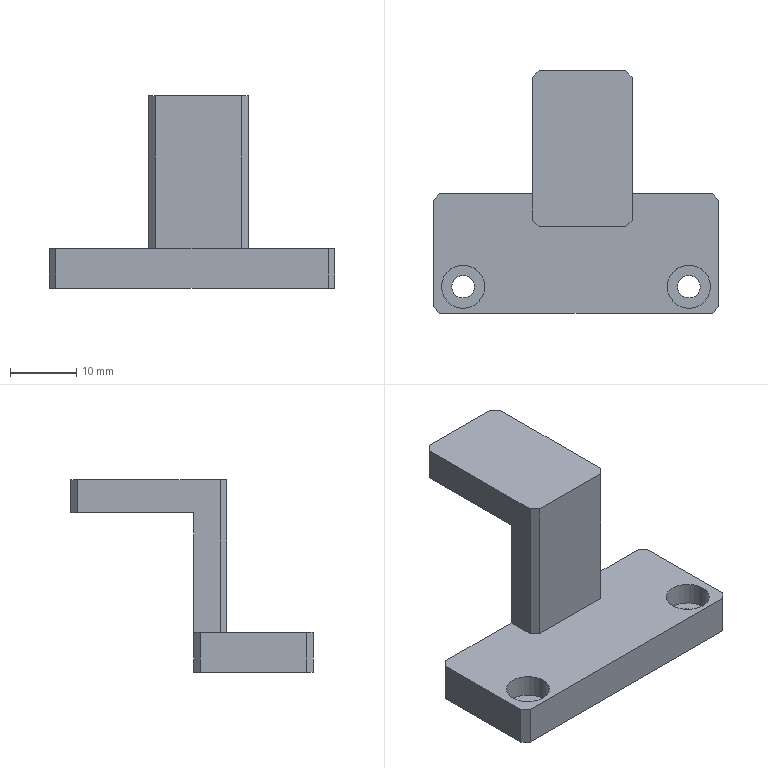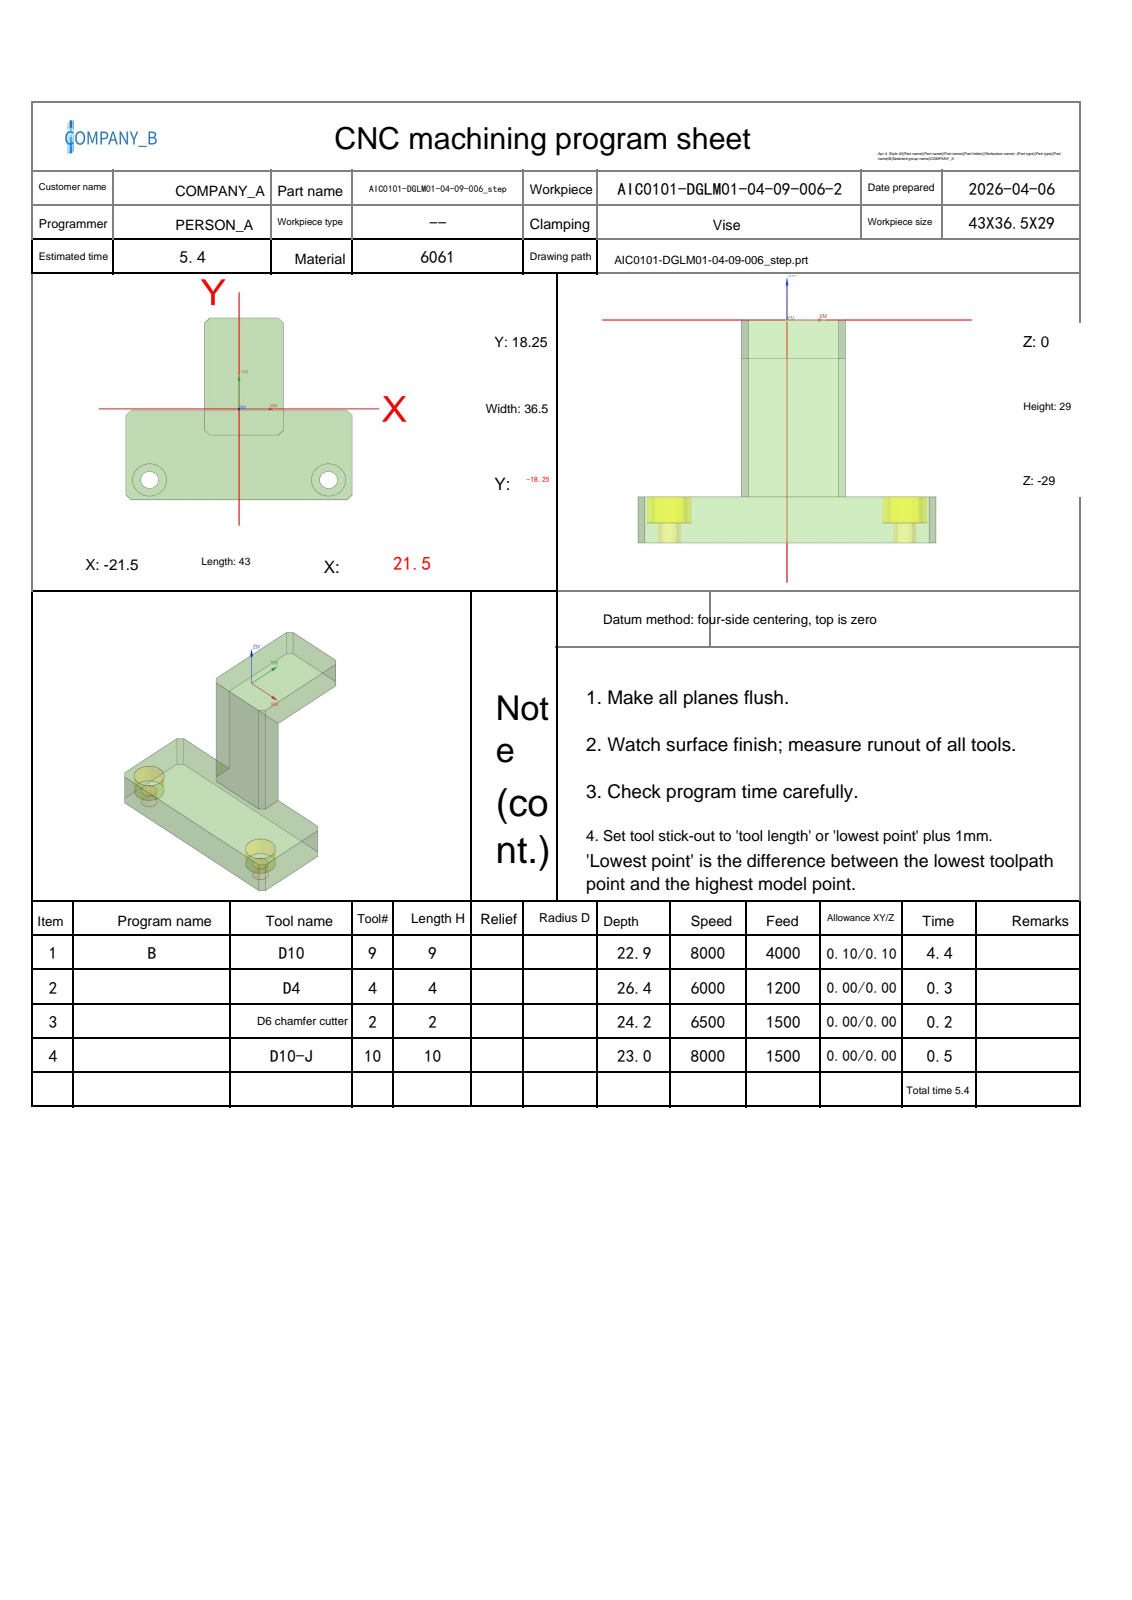NC program | NX | posted by the shop | part box 43 x 36.5 x 29 mm
Lines 1 to 972 of 4586:
%
O0001
(Machine time: 6.22 MIN)
(===Total Tool:4===)
(T9=D10     D=10.  R=0.   D-  H09 Z=-22.9 )
(T4=D4      D=4.   R=0.   D-  H04 Z=-26.4 )
(T2=D6 chamfer cutter   D=6.   R=0.   D-  H02 Z=-24.2 )
(T10=D10-J  D=10.  R=0.   D10 H10 Z=-23.  )
G80 G90 G17 G49 G40
G91 G28 Z0
M01
N1 T09 M06
(D10  D=10. R=0. H=09 ce=0.25 di=0.10)
G00 G90 G54 X-35.099 Y-10.332 M03 S8000
G43 H09 Z20.
M08
Z2.1
G01 X-35.001 Y-10.314 Z1.476 F4000.
X-34.903 Y-10.296 Z1.228
X-34.804 Y-10.278 Z1.046
X-34.706 Y-10.26 Z.9
X-34.607 Y-10.242 Z.777
X-34.509 Y-10.224 Z.672
X-34.411 Y-10.206 Z.58
X-34.312 Y-10.188 Z.5
X-34.214 Y-10.17 Z.43
X-34.116 Y-10.152 Z.368
X-34.017 Y-10.134 Z.314
X-33.919 Y-10.116 Z.267
X-33.82 Y-10.098 Z.227
X-33.722 Y-10.08 Z.192
X-33.624 Y-10.062 Z.164
X-33.525 Y-10.044 Z.14
X-33.427 Y-10.027 Z.123
X-33.329 Y-10.009 Z.11
X-33.23 Y-9.991 Z.103
X-33.132 Y-9.973 Z.1
X-30.88 Y-9.561
G03 X-30.51 Y-9.27 I-.096 J.503
X-29.9 Y-6.027 I-9.761 J3.513
X-29.692 Y2.334 I-167.742 J8.361
X-29.702 Y4.201 I-167.951 J0.0
G02 X-29.723 Y9.588 I703.046 J5.387
X-29.664 Y18.677 I703.067 J0.0
X-25.831 Y24.268 I6.588 J-.408
X-19.878 Y25.71 I6.684 J-14.582
X-11.771 Y25.954 I8.107 J-135.053
X-10.284 Y25.945 I0.0 J-135.296
G01 X22.13 Y25.932
G02 X28.067 Y21.993 I-.133 J-6.643
X29.449 Y16.271 I-14.607 J-6.557
X29.713 Y7.575 I-143.052 J-8.695
X29.698 Y5.476 I-143.316 J0.0
G01 X29.681 Y-18.42
G02 X25.869 Y-24.247 I-6.599 J.158
X20.079 Y-25.692 I-6.608 J14.146
X11.869 Y-25.956 I-8.21 J127.869
X10.245 Y-25.945 I0.0 J128.132
G01 X-22.171 Y-25.93
G02 X-28.026 Y-22.061 I.169 J6.619
X-29.462 Y-16.11 I14.613 J6.676
X-29.614 Y-12.83 I35.28 J3.28
X-29.302 Y-8.137 I35.432 J0.0
G03 X-28.904 Y2.261 I-135.723 J10.398
X-28.91 Y3.491 I-136.121 J0.0
G02 X-28.922 Y7.625 I709.413 J4.134
X-28.863 Y16.738 I709.425 J0.0
X-24.741 Y22.947 I7.759 J-.678
X-18.641 Y24.75 I7.505 J-14.175
X-10.084 Y25.147 I8.556 J-91.966
X-8.813 Y25.138 I0.0 J-92.364
G01 X20.207 Y25.129
G02 X26.68 Y21.024 I-.379 J-7.754
X28.524 Y14.687 I-14.343 J-7.61
X28.906 Y5.741 I-104.616 J-8.946
X28.893 Y4.059 I-104.998 J0.0
G01 X28.882 Y-16.417
G02 X24.804 Y-22.91 I-7.753 J.342
X18.39 Y-24.779 I-7.66 J14.347
X9.425 Y-25.156 I-8.965 J106.528
X7.761 Y-25.143 I0.0 J106.905
G01 X-20.167 Y-25.131
G02 X-26.629 Y-21.102 I.341 J7.744
X-28.535 Y-14.46 I14.057 J7.628
X-28.605 Y-11.776 I51.743 J2.683
X-28.407 Y-7.251 I51.812 J0.0
G03 X-28.081 Y7.217 I-320.735 J14.467
X-28.101 Y10.838 I-321.061 J0.0
G02 X-28.126 Y12.212 I38.122 J1.374
X-27.974 Y15.613 I38.147 J0.0
X-23.079 Y22.154 I8.78 J-1.468
X-16.395 Y23.964 I8.13 J-16.776
X-7.027 Y24.352 I9.368 J-112.703
X-5.446 Y24.341 I0.0 J-113.092
G01 X18.294 Y24.327
G02 X25.851 Y19.431 I-.359 J-8.835
X27.7 Y12.764 I-16.412 J-8.143
X28.105 Y3.246 I-111.872 J-9.518
X28.092 Y1.576 I-112.276 J0.0
X28.118 Y-5.22 I-878.703 J-6.795
X28.067 Y-14.723 I-878.729 J0.0
X23.208 Y-22.083 I-8.816 J.536
X16.623 Y-23.937 I-8.116 J16.208
X7.487 Y-24.347 I-9.136 J101.66
X6.156 Y-24.338 I0.0 J102.07
G01 X-18.144 Y-24.333
G02 X-25.822 Y-19.476 I.219 J8.843
X-27.593 Y-12.229 I14.676 J7.426
X-27.611 Y-10.065 I128.798 J2.164
X-27.441 Y-3.447 I128.816 J0.0
G03 X-27.276 Y12.759 I-867.03 J16.931
G02 X-21.723 Y21.294 I9.672 J-.219
X-14.557 Y23.163 I8.645 J-18.474
X-4.967 Y23.548 I9.59 J-119.225
X-3.528 Y23.539 I0.0 J-119.61
G01 X16.532 Y23.523
G02 X25.055 Y17.953 I-.24 J-9.674
X26.881 Y11.109 I-18.139 J-8.505
X27.3 Y1.375 I-112.809 J-9.735
X27.289 Y-.158 I-113.228 J0.0
X27.307 Y-5.158 I-719.586 J-4.999
X27.265 Y-12.938 I-719.603 J0.0
X21.676 Y-21.318 I-9.667 J.393
X14.669 Y-23.151 I-8.567 J18.443
X5.031 Y-23.548 I-9.638 J116.603
X3.561 Y-23.539 I0.0 J117.
G01 X-16.259 Y-23.534
X-16.273
G02 X-25.201 Y-17.597 I0.0 J9.682
X-26.646 Y-10.669 I17.356 J7.235
X-26.685 Y-6.775 I195.538 J3.894
X-26.569 Y-.062 I195.577 J0.0
X-26.455 Y11.482 I890.841 J-3.088
X-20.487 Y20.435 I10.294 J-.397
X-13.408 Y22.308 I8.863 J-19.183
X-3.331 Y22.748 I10.076 J-115.189
X-1.821 Y22.738 I0.0 J-115.629
X5.249 Y22.767 I7.07 J-872.675
X15.038 Y22.712 I0.0 J-872.703
X24.267 Y16.57 I-.229 J-10.348
X26.096 Y9.315 I-20.036 J-8.91
X26.496 Y-.533 I-121.222 J-9.847
X26.488 Y-1.874 I-121.622 J0.0
X26.517 Y-5.594 I-238.869 J-3.72
X26.441 Y-11.633 I-238.898 J0.0
X20.365 Y-20.493 I-10.296 J.547
X12.873 Y-22.365 I-9.019 J20.176
X3.265 Y-22.742 I-9.608 J122.293
X2.164 Y-22.737 I0.0 J122.67
X-5.189 Y-22.767 I-7.352 J884.922
X-15.016 Y-22.713 I0.0 J884.953
X-24.356 Y-16.185 I.158 J10.172
X-25.751 Y-8.916 I20.041 J7.614
X-25.817 Y-3.574 I217.316 J5.341
X-25.743 Y2.076 I217.381 J0.0
X-25.745 Y3.097 I237.464 J1.02
X-25.639 Y10.209 I237.467 J0.0
X-19.185 Y19.649 I10.846 J-.489
X-11.532 Y21.546 I9.29 J-21.093
X-1.516 Y21.942 I10.015 J-126.302
X-.262 Y21.936 I0.0 J-126.699
X5.345 Y21.967 I5.607 J-504.237
X13.717 Y21.898 I0.0 J-504.268
X23.33 Y15.576 I-.237 J-10.831
X25.263 Y8.097 I-20.328 J-9.243
X25.695 Y-2.142 I-121.077 J-10.24
X25.687 Y-3.57 I-121.509 J0.0
X25.716 Y-5.906 I-93.971 J-2.336
X25.598 Y-10.608 I-94. J0.0
X19.283 Y-19.599 I-10.758 J.843
X11.718 Y-21.526 I-9.272 J20.586
X1.596 Y-21.944 I-10.122 J122.471
X.29 Y-21.937 I0.0 J122.889
X-5.352 Y-21.971 I-5.642 J461.8
X-13.769 Y-21.894 I0.0 J461.834
X-23.383 Y-15.145 I.225 J10.543
X-24.839 Y-8.041 I20.527 J7.907
X-24.983 Y-1.004 I171.254 J7.037
X-24.934 Y3.106 I171.399 J0.0
X-24.945 Y4.407 I78.052 J1.301
X-24.779 Y9.493 I78.063 J0.0
X-18.144 Y18.768 I11.205 J-1.005
X-10.583 Y20.695 I9.454 J-21.297
X-.124 Y21.143 I10.459 J-121.839
X1.244 Y21.135 I0.0 J-122.287
X5.457 Y21.162 I4.213 J-334.395
X12.363 Y21.091 I0.0 J-334.422
X20.144 Y17.822 I-.204 J-11.382
X23.766 Y10.832 I-10.854 J-10.057
X24.783 Y1.624 I-44.86 J-9.611
X24.898 Y-4.053 I-139.858 J-5.677
X24.81 Y-9.014 I-139.973 J0.0
X18.124 Y-18.775 I-11.253 J.538
X10.323 Y-20.722 I-9.548 J21.645
X-.202 Y-21.145 I-10.525 J130.707
X-1.665 Y-21.137 I0.0 J131.13
X-5.681 Y-21.166 I-4.016 J280.073
X-12.464 Y-21.084 I0.0 J280.102
X-19.777 Y-18.098 I.247 J11.055
X-23.319 Y-11.371 I9.676 J9.39
X-24.126 Y-3.277 I40.22 J8.094
X-24.123 Y-2.784 I41.026 J0.0
X-24.159 Y.812 I179.52 J3.597
X-24.027 Y7.673 I179.556 J0.0
X-19.342 Y16.576 I11.625 J-.434
X-12.27 Y19.446 I9.931 J-14.322
X-2.397 Y20.273 I9.913 J-58.987
X4.527 Y20.359 I6.924 J-277.627
X11.122 Y20.281 I0.0 J-277.713
X18.549 Y17.514 I-.247 J-12.017
X22.677 Y10.666 I-9.496 J-10.391
X23.917 Y1.813 I-37.219 J-9.726
X24.074 Y-3.664 I-95.415 J-5.477
X23.978 Y-7.942 I-95.573 J0.0
X17.054 Y-17.93 I-11.608 J.654
X9.251 Y-19.892 I-9.705 J22.092
X-1.267 Y-20.339 I-10.518 J123.549
X-2.496 Y-20.333 I0.0 J123.996
X-5.605 Y-20.36 I-3.11 J178.005
X-11.294 Y-20.269 I0.0 J178.033
X-18.637 Y-17.327 I.323 J11.44
X-22.346 Y-10.607 I9.587 J9.674
X-23.277 Y-2.129 I38.123 J8.478
G01 Y-2.036
G02 X-23.338 Y1.46 I99.559 J3.496
X-23.197 Y6.76 I99.621 J0.0
X-15.895 Y17.151 I12.014 J-.682
X-8. Y19.088 I9.877 J-23.198
X2.785 Y19.539 I10.785 J-128.663
X4.067 Y19.533 I0.0 J-129.115
X6.025 Y19.561 I1.958 J-68.354
X10.942 Y19.384 I0.0 J-68.382
X20.81 Y12.331 I-1.038 J-11.884
X22.824 Y4.381 I-22.519 J-9.935
X23.23 Y-3.317 I-72.836 J-7.699
X23.147 Y-6.803 I-73.242 J0.0
X15.953 Y-17.119 I-11.932 J.655
X7.751 Y-19.113 I-10.029 J23.382
X-3.155 Y-19.543 I-10.905 J138.046
X-4.638 Y-19.535 I0.0 J138.476
X-6.396 Y-19.565 I-1.758 J52.38
X-11.349 Y-19.33 I0.0 J52.409
X-20.515 Y-12.319 I1.4 J11.327
X-22.266 Y-4.388 I22.554 J9.139
X-22.504 Y1.323 I68.472 J5.711
X-22.344 Y6.002 I68.709 J0.0
X-15.122 Y16.202 I12.194 J-.977
X-7.098 Y18.251 I10.109 J-22.851
X4.217 Y18.743 I11.315 J-129.888
X6.007 Y18.731 I0.0 J-130.38
X6.856 Y18.746 I.849 J-23.129
X12.197 Y18.122 I0.0 J-23.144
X19.962 Y11.346 I-3.378 J-11.707
X22.014 Y3.24 I-23.024 J-10.141
X22.372 Y-2.804 I-50.768 J-6.044
X22.265 Y-6.104 I-51.126 J0.0
X15.188 Y-16.162 I-12.056 J.964
X7.006 Y-18.261 I-10.19 J22.724
X-4.228 Y-18.743 I-11.233 J130.707
X-6.02 Y-18.73 I0.0 J131.189
X-6.851 Y-18.746 I-.831 J22.555
X-12.052 Y-18.138 I0.0 J22.571
X-19.617 Y-11.346 I3.255 J11.234
X-21.391 Y-3.663 I22.516 J9.245
X-21.643 Y1.253 I47.658 J4.916
X-21.48 Y5.204 I47.91 J0.0
X-14.139 Y15.365 I12.368 J-1.203
X-5.959 Y17.445 I10.291 J-23.354
X3.731 Y17.909 I9.689 J-100.918
X8.025 Y17.818 I0.0 J-101.382
X15.743 Y14.883 I-.511 J-12.961
X20.159 Y7.634 I-9.99 J-11.055
X21.484 Y-2.348 I-36.948 J-9.982
X21.359 Y-5.445 I-38.272 J0.0
X14.277 Y-15.286 I-12.169 J1.288
X6.108 Y-17.427 I-10.304 J22.663
X-3.714 Y-17.908 I-9.822 J99.91
X-7.954 Y-17.819 I0.0 J100.392
X-15.568 Y-14.827 I.475 J12.39
X-19.659 Y-7.771 I9.912 J10.461
X-20.754 Y.988 I34.486 J8.758
X-20.56 Y4.691 I35.581 J0.0
X-13.38 Y14.43 I12.399 J-1.625
X-5.297 Y16.587 I10.395 J-22.731
X3.288 Y17.073 I8.585 J-75.618
X7.243 Y16.97 I0.0 J-76.104
X15.566 Y13.339 I-.659 J-12.866
X19.508 Y6.025 I-11.673 J-11.009
X20.559 Y-2.044 I-30.451 J-8.069
X20.467 Y-4.442 I-31.502 J0.0
X13.343 Y-14.43 I-12.266 J1.215
X5.34 Y-16.58 I-10.336 J22.504
X-3.264 Y-17.072 I-8.605 J75.058
X-7.119 Y-16.973 I0.0 J75.55
X-15.378 Y-13.222 I.611 J12.311
X-19.008 Y-5.979 I11.796 J10.444
X-19.822 Y.763 I27.522 J6.742
X-19.643 Y3.949 I28.336 J0.0
X-12.607 Y13.505 I12.403 J-1.764
X-4.393 Y15.76 I10.579 J-22.45
X2.907 Y16.219 I7.3 J-57.794
X6.466 Y16.11 I0.0 J-58.254
X17.471 Y8.416 I-.795 J-12.856
X19.595 Y-1.634 I-22.721 J-10.05
X19.496 Y-3.849 I-24.844 J0.0
X12.709 Y-13.427 I-12.172 J1.431
X4.669 Y-15.722 I-10.509 J21.591
X-2.814 Y-16.218 I-7.483 J56.159
X-6.426 Y-16.103 I0.0 J56.655
X-16.985 Y-8.499 I.89 J12.369
X-18.846 Y.514 I20.904 J9.013
X-18.672 Y3.321 I22.764 J0.0
X-11.746 Y12.627 I12.335 J-1.949
X-3.383 Y14.948 I10.737 J-22.464
X2.469 Y15.349 I5.852 J-42.537
X6.035 Y15.2 I0.0 J-42.938
X16.553 Y7.66 I-1.251 J-12.851
X18.578 Y-1.232 I-18.506 J-8.892
X18.464 Y-3.4 I-20.532 J0.0
X11.922 Y-12.498 I-12.014 J1.738
X3.831 Y-14.885 I-10.633 J21.134
X-2.443 Y-15.342 I-6.274 J42.853
X-5.663 Y-15.222 I0.0 J43.31
X-16.09 Y-7.637 I1.091 J12.459
X-17.813 Y.221 I17.062 J7.858
X-17.619 Y2.911 I18.785 J0.0
X-10.945 Y11.719 I12.145 J-2.271
X-2.837 Y14.077 I10.705 J-21.685
X2.074 Y14.454 I4.911 J-31.865
X5.696 Y14.25 I0.0 J-32.242
X15.747 Y6.678 I-1.787 J-12.83
X17.507 Y-.908 I-15.47 J-7.586
X17.41 Y-2.73 I-17.23 J0.0
X11.152 Y-11.555 I-11.804 J1.739
X3.089 Y-14.035 I-10.693 J20.422
X-2.002 Y-14.442 I-5.092 J31.603
X-5.283 Y-14.274 I0.0 J32.01
X-15.202 Y-6.766 I1.598 J12.417
X-16.717 Y-.075 I14.013 J6.691
X-16.472 Y2.673 I15.529 J0.0
X-10.294 Y10.72 I11.802 J-2.666
X-1.917 Y13.248 I10.825 J-20.726
X1.731 Y13.533 I3.647 J-23.19
X5.807 Y13.177 I0.0 J-23.475
X14.889 Y5.788 I-2.708 J-12.604
X16.363 Y-.467 I-12.53 J-6.255
X16.144 Y-2.934 I-14.005 J0.0
X10.318 Y-10.636 I-11.422 J2.586
X2.282 Y-13.188 I-10.653 J19.622
X-1.579 Y-13.515 I-3.861 J22.573
X-5.441 Y-13.187 I0.0 J22.901
X-14.402 Y-5.664 I2.585 J12.178
X-15.552 Y-.408 I11.441 J5.256
X-14.965 Y3.392 I12.591 J0.0
X-8.808 Y10.164 I11.459 J-4.232
X1.477 Y12.541 I10.285 J-21.074
X4.266 Y12.374 I0.0 J-23.45
X14.431 Y3.836 I-1.92 J-12.606
X15.16 Y-.086 I-10.183 J-3.922
X10.235 Y-9.209 I-10.913 J0.0
X2.043 Y-12.235 I-10.749 J16.5
X-1.244 Y-12.539 I-3.287 J17.633
X-5.497 Y-12.027 I0.0 J17.936
X-14.275 Y-.439 I3.26 J11.588
X-14.213 Y.775 I12.038 J0.0
X-9.045 Y8.606 I10.962 J-1.613
X1.189 Y11.519 I10.235 J-16.523
X3.765 Y11.348 I0.0 J-19.436
X13.808 Y.656 I-1.729 J-11.687
X13.817 Y.229 I-10.242 J-.426
X9.582 Y-8.071 I-10.251 J0.0
X.689 Y-11.391 I-10.498 J14.548
X-1.122 Y-11.517 I-1.81 J12.935
X-7.568 Y-9.815 I0.0 J13.061
X-12.912 Y-.645 I5.365 J9.268
X-8.602 Y7.326 I10.217 J-.372
X.923 Y10.433 I9.525 J-13.049
X3.471 Y10.231 I0.0 J-16.156
X11.94 Y3.058 I-1.82 J-10.736
X12.341 Y.368 I-8.818 J-2.69
X9.443 Y-6.343 I-9.219 J0.0
X.292 Y-10.333 I-10.199 J10.901
X-.936 Y-10.401 I-1.228 J11.081
X-9.056 Y-6.892 I0.0 J11.148
X-11.361 Y-.964 I6.47 J5.928
X-8.968 Y5.059 I8.775 J0.0
X.674 Y9.262 I9.642 J-8.958
X3.721 Y8.905 I0.0 J-13.161
X10.164 Y3.498 I-2.189 J-9.152
X10.705 Y.539 I-7.827 J-2.959
X8.359 Y-5.271 I-8.368 J0.0
X-.504 Y-9.135 I-8.862 J8.231
X-3.266 Y-8.816 I0.0 J12.095
X-9.231 Y-3.597 I1.892 J8.182
X-9.613 Y-1.14 I7.711 J2.457
X-7.269 Y4.557 I8.093 J0.0
X.524 Y7.955 I7.793 J-7.237
X3.921 Y7.398 I0.0 J-10.635
X8.829 Y.614 I-2.235 J-6.784
G01 Y.592
G02 X4.759 Y-6.202 I-8.392 J.412
X-.297 Y-7.736 I-5.056 J7.568
X-3.736 Y-7.061 I0.0 J9.101
X-7.557 Y-1.158 I2.649 J5.903
X-6.776 Y1.925 I6.47 J0.0
X.42 Y6.357 I7.196 J-3.626
X2.264 Y6.143 I0.0 J-8.058
X6.402 Y.697 I-1.515 J-5.446
X5.99 Y-1.421 I-5.653 J0.0
X.012 Y-5.749 I-6.145 J2.195
X-4.292 Y-1.308 I.139 J4.441
X-3.901 Y.516 I4.443 J0.0
G01 X-3.376 Y1.594
X-3.33 Y1.683 Z.103
X-3.284 Y1.772 Z.11
X-3.238 Y1.861 Z.123
X-3.192 Y1.949 Z.14
X-3.146 Y2.038 Z.164
X-3.1 Y2.127 Z.192
X-3.054 Y2.216 Z.227
X-3.008 Y2.305 Z.267
X-2.962 Y2.393 Z.314
X-2.916 Y2.482 Z.368
X-2.87 Y2.571 Z.43
X-2.824 Y2.66 Z.5
X-2.778 Y2.749 Z.58
X-2.732 Y2.837 Z.672
X-2.686 Y2.926 Z.777
X-2.64 Y3.015 Z.9
X-2.594 Y3.104 Z1.046
X-2.548 Y3.193 Z1.228
X-2.502 Y3.281 Z1.476
X-2.456 Y3.37 Z2.1
G00 Z20.
G00 G90 X-16.642 Y-26.25 M03 S8000
Z15.5
Z.913
G01 Z-.587 F4000.
Y-23.15
X-22.53
X-23.965 Y-21.715
X-26.4 Y-19.28
Y.78
X-22.53 Y4.65
X-15.949
X-15.863 Y4.653
X-15.804 Y4.589
X-15.661 Y4.444
G03 X-15.464 Y4.349 I.23 J.227
G02 X-13.22 Y1.863 I-.256 J-2.487
X-13.415 Y.894 I-2.5 J0.0
G01 X-17.755 Y-9.432
G02 X-20.06 Y-10.963 I-2.305 J.969
X-22.56 Y-8.463 I0.0 J2.5
X-22.365 Y-7.495 I2.5 J0.0
G01 X-18.025 Y2.831
G02 X-15.938 Y4.353 I2.305 J-.969
G01 X-15.86 Y4.354
X-15.81 Y4.413
X-15.674 Y4.551
G02 X-15.437 Y4.65 I.237 J-.233
G01 X-11.65
Y-6.362
X-7.662 Y-10.35
X9.562
X13.55 Y-6.362
Y4.65
X18.043
X18.087 Y4.661
X18.111 Y4.622
X18.175 Y4.557
X18.212 Y4.508
X18.274 Y4.513
G02 X20.615 Y2.433 I-.124 J-2.497
G01 X22.774 Y-10.329
G02 X22.809 Y-10.746 I-2.465 J-.417
X20.309 Y-13.246 I-2.5 J0.0
X17.844 Y-11.163 I0.0 J2.5
G01 X15.685 Y1.599
G02 X15.65 Y2.016 I2.465 J.417
X18.046 Y4.514 I2.5 J0.0
G01 X18.088 Y4.504
X18.109 Y4.542
X18.172 Y4.605
X18.214 Y4.657
X18.28 Y4.65
X22.53
X26.4 Y.78
Y-19.28
X22.53 Y-23.15
X20.502
G02 X19.554 Y-22.467 I0.0 J1.
G01 X17.457 Y-16.177
G03 X16.896 Y-15.572 I-.949 J-.317
G02 X16.283 Y-14.65 I.387 J.922
X16.575 Y-13.944 I1. J0.0
G01 X17.194 Y-13.325
G02 X17.9 Y-13.033 I.706 J-.708
X18.9 Y-14.032 I0.0 J-1.
G01 Y-14.652
G02 X18.262 Y-15.582 I-1. J.002
G03 X17.702 Y-16.129 I.363 J-.932
G01 X15.038 Y-22.535
G02 X14.115 Y-23.15 I-.923 J.385
G01 X-9.665
G02 X-10.446 Y-22.774 I0.0 J1.
G01 X-13.891 Y-18.459
X-13.947 Y-18.395
G02 X-14.635 Y-16.673 I1.812 J1.722
X-12.135 Y-14.173 I2.5 J0.0
G01 X14.035
G02 X16.535 Y-16.673 I0.0 J-2.5
X14.035 Y-19.173 I-2.5 J0.0
G01 X-9.655
G03 X-10.446 Y-19.562 I0.0 J-1.
G01 X-12.564 Y-22.307
G02 X-14.28 Y-23.15 I-1.715 J1.324
G01 X-14.39
G02 X-14.677 Y-22.962 I0.0 J.315
G01 X-17.696 Y-16.116
G03 X-18.255 Y-15.585 I-.915 J-.404
G02 X-18.9 Y-14.652 I.355 J.935
G01 Y-12.122
G02 X-17.9 Y-11.123 I1. J-.002
X-17.166 Y-11.444 I0.0 J-1.
G03 X-16.953 Y-11.666 I5.516 J5.082
G01 X-14.675 Y-13.944
G02 X-14.383 Y-14.65 I-.708 J-.706
X-15.382 Y-15.65 I-1. J0.0
G01 X-15.882
Y-26.25
Z.913
G00 X-16.642
Z.326
G01 Z-1.174
Y-23.15
X-22.53
X-23.965 Y-21.715
X-26.4 Y-19.28
Y.78
X-22.53 Y4.65
X-15.949
X-15.863 Y4.653
X-15.804 Y4.589
X-15.661 Y4.444
G03 X-15.464 Y4.349 I.23 J.227
G02 X-13.22 Y1.863 I-.256 J-2.487
X-13.415 Y.894 I-2.5 J0.0
G01 X-17.755 Y-9.432
G02 X-20.06 Y-10.963 I-2.305 J.969
X-22.56 Y-8.463 I0.0 J2.5
X-22.365 Y-7.495 I2.5 J0.0
G01 X-18.025 Y2.831
G02 X-15.938 Y4.353 I2.305 J-.969
G01 X-15.86 Y4.354
X-15.81 Y4.413
X-15.674 Y4.551
G02 X-15.437 Y4.65 I.237 J-.233
G01 X-11.65
Y-6.362
X-7.662 Y-10.35
X9.562
X13.55 Y-6.362
Y4.65
X18.043
X18.087 Y4.661
X18.111 Y4.622
X18.175 Y4.557
X18.212 Y4.508
X18.274 Y4.513
G02 X20.615 Y2.433 I-.124 J-2.497
G01 X22.774 Y-10.329
G02 X22.809 Y-10.746 I-2.465 J-.417
X20.309 Y-13.246 I-2.5 J0.0
X17.844 Y-11.163 I0.0 J2.5
G01 X15.685 Y1.599
G02 X15.65 Y2.016 I2.465 J.417
X18.046 Y4.514 I2.5 J0.0
G01 X18.088 Y4.504
X18.109 Y4.542
X18.172 Y4.605
X18.214 Y4.657
X18.28 Y4.65
X22.53
X26.4 Y.78
Y-19.28
X22.53 Y-23.15
X20.502
G02 X19.554 Y-22.467 I0.0 J1.
G01 X17.457 Y-16.177
G03 X16.896 Y-15.572 I-.949 J-.317
G02 X16.283 Y-14.65 I.387 J.922
X16.575 Y-13.944 I1. J0.0
G01 X17.194 Y-13.325
G02 X17.9 Y-13.033 I.706 J-.708
X18.9 Y-14.032 I0.0 J-1.
G01 Y-14.652
G02 X18.262 Y-15.582 I-1. J.002
G03 X17.702 Y-16.129 I.363 J-.932
G01 X15.038 Y-22.535
G02 X14.115 Y-23.15 I-.923 J.385
G01 X-9.665
G02 X-10.446 Y-22.774 I0.0 J1.
G01 X-13.891 Y-18.459
X-13.947 Y-18.395
G02 X-14.635 Y-16.673 I1.812 J1.722
X-12.135 Y-14.173 I2.5 J0.0
G01 X14.035
G02 X16.535 Y-16.673 I0.0 J-2.5
X14.035 Y-19.173 I-2.5 J0.0
G01 X-9.655
G03 X-10.446 Y-19.562 I0.0 J-1.
G01 X-12.564 Y-22.307
G02 X-14.28 Y-23.15 I-1.715 J1.324
G01 X-14.39
G02 X-14.677 Y-22.962 I0.0 J.315
G01 X-17.696 Y-16.116
G03 X-18.255 Y-15.585 I-.915 J-.404
G02 X-18.9 Y-14.652 I.355 J.935
G01 Y-12.122
G02 X-17.9 Y-11.123 I1. J-.002
X-17.166 Y-11.444 I0.0 J-1.
G03 X-16.953 Y-11.666 I5.516 J5.082
G01 X-14.675 Y-13.944
G02 X-14.383 Y-14.65 I-.708 J-.706
X-15.382 Y-15.65 I-1. J0.0
G01 X-15.882
Y-26.25
Z.326
G00 X-16.642
Z-.262
G01 Z-1.762
Y-23.15
X-22.53
X-23.965 Y-21.715
X-26.4 Y-19.28
Y.78
X-22.53 Y4.65
X-15.949
X-15.863 Y4.653
X-15.804 Y4.589
X-15.661 Y4.444
G03 X-15.464 Y4.349 I.23 J.227
G02 X-13.22 Y1.863 I-.256 J-2.487
X-13.415 Y.894 I-2.5 J0.0
G01 X-17.755 Y-9.432
G02 X-20.06 Y-10.963 I-2.305 J.969
X-22.56 Y-8.463 I0.0 J2.5
X-22.365 Y-7.495 I2.5 J0.0
G01 X-18.025 Y2.831
G02 X-15.938 Y4.353 I2.305 J-.969
G01 X-15.86 Y4.354
X-15.81 Y4.413
X-15.674 Y4.551
G02 X-15.437 Y4.65 I.237 J-.233
G01 X-11.65
Y-6.362
X-7.662 Y-10.35
X9.562
X13.55 Y-6.362
Y4.65
X18.043
X18.087 Y4.661
X18.111 Y4.622
X18.175 Y4.557
X18.212 Y4.508
X18.274 Y4.513
G02 X20.615 Y2.433 I-.124 J-2.497
G01 X22.774 Y-10.329
G02 X22.809 Y-10.746 I-2.465 J-.417
X20.309 Y-13.246 I-2.5 J0.0
X17.844 Y-11.163 I0.0 J2.5
G01 X15.685 Y1.599
G02 X15.65 Y2.016 I2.465 J.417
X18.046 Y4.514 I2.5 J0.0
G01 X18.088 Y4.504
X18.109 Y4.542
X18.172 Y4.605
X18.214 Y4.657
X18.28 Y4.65
X22.53
X26.4 Y.78
Y-19.28
X22.53 Y-23.15
X20.502
G02 X19.554 Y-22.467 I0.0 J1.
G01 X17.457 Y-16.177
G03 X16.896 Y-15.572 I-.949 J-.317
G02 X16.283 Y-14.65 I.387 J.922
X16.575 Y-13.944 I1. J0.0
G01 X17.194 Y-13.325
G02 X17.9 Y-13.033 I.706 J-.708
X18.9 Y-14.032 I0.0 J-1.
G01 Y-14.652
G02 X18.262 Y-15.582 I-1. J.002
G03 X17.702 Y-16.129 I.363 J-.932
G01 X15.038 Y-22.535
G02 X14.115 Y-23.15 I-.923 J.385
G01 X-9.665
G02 X-10.446 Y-22.774 I0.0 J1.
G01 X-13.891 Y-18.459
X-13.947 Y-18.395
G02 X-14.635 Y-16.673 I1.812 J1.722
X-12.135 Y-14.173 I2.5 J0.0
G01 X14.035
G02 X16.535 Y-16.673 I0.0 J-2.5
X14.035 Y-19.173 I-2.5 J0.0
G01 X-9.655
G03 X-10.446 Y-19.562 I0.0 J-1.
G01 X-12.564 Y-22.307
G02 X-14.28 Y-23.15 I-1.715 J1.324
G01 X-14.39
G02 X-14.677 Y-22.962 I0.0 J.315
G01 X-17.696 Y-16.116
G03 X-18.255 Y-15.585 I-.915 J-.404
G02 X-18.9 Y-14.652 I.355 J.935
G01 Y-12.122
G02 X-17.9 Y-11.123 I1. J-.002
X-17.166 Y-11.444 I0.0 J-1.
G03 X-16.953 Y-11.666 I5.516 J5.082
G01 X-14.675 Y-13.944
G02 X-14.383 Y-14.65 I-.708 J-.706
X-15.382 Y-15.65 I-1. J0.0
G01 X-15.882
Y-26.25
Z-.262
G00 X-16.642
Z-.849
G01 Z-2.349
Y-23.15
X-22.53
X-23.965 Y-21.715
X-26.4 Y-19.28
Y.78
X-22.53 Y4.65
X-15.949
X-15.863 Y4.653
X-15.804 Y4.589
X-15.661 Y4.444
G03 X-15.464 Y4.349 I.23 J.227
G02 X-13.22 Y1.863 I-.256 J-2.487
X-13.415 Y.894 I-2.5 J0.0
G01 X-17.755 Y-9.432
G02 X-20.06 Y-10.963 I-2.305 J.969
X-22.56 Y-8.463 I0.0 J2.5
X-22.365 Y-7.495 I2.5 J0.0
G01 X-18.025 Y2.831
G02 X-15.938 Y4.353 I2.305 J-.969
G01 X-15.86 Y4.354
X-15.81 Y4.413
X-15.674 Y4.551
G02 X-15.437 Y4.65 I.237 J-.233
G01 X-11.65
Y-6.362
X-7.662 Y-10.35
X9.562
X13.55 Y-6.362
Y4.65
X18.043
X18.087 Y4.661
X18.111 Y4.622
X18.175 Y4.557
X18.212 Y4.508
X18.274 Y4.513
G02 X20.615 Y2.433 I-.124 J-2.497
G01 X22.774 Y-10.329
G02 X22.809 Y-10.746 I-2.465 J-.417
X20.309 Y-13.246 I-2.5 J0.0
X17.844 Y-11.163 I0.0 J2.5
G01 X15.685 Y1.599
G02 X15.65 Y2.016 I2.465 J.417
X18.046 Y4.514 I2.5 J0.0
G01 X18.088 Y4.504
X18.109 Y4.542
X18.172 Y4.605
X18.214 Y4.657
X18.28 Y4.65
X22.53
X26.4 Y.78
Y-19.28
X22.53 Y-23.15
X20.502
G02 X19.554 Y-22.467 I0.0 J1.
G01 X17.457 Y-16.177
G03 X16.896 Y-15.572 I-.949 J-.317
G02 X16.283 Y-14.65 I.387 J.922
X16.575 Y-13.944 I1. J0.0
G01 X17.194 Y-13.325
G02 X17.9 Y-13.033 I.706 J-.708
X18.9 Y-14.032 I0.0 J-1.
G01 Y-14.652
G02 X18.262 Y-15.582 I-1. J.002
G03 X17.702 Y-16.129 I.363 J-.932
G01 X15.038 Y-22.535
G02 X14.115 Y-23.15 I-.923 J.385
G01 X-9.665
G02 X-10.446 Y-22.774 I0.0 J1.
G01 X-13.891 Y-18.459
X-13.947 Y-18.395
G02 X-14.635 Y-16.673 I1.812 J1.722
X-12.135 Y-14.173 I2.5 J0.0
G01 X14.035
G02 X16.535 Y-16.673 I0.0 J-2.5
X14.035 Y-19.173 I-2.5 J0.0
G01 X-9.655
G03 X-10.446 Y-19.562 I0.0 J-1.
G01 X-12.564 Y-22.307
G02 X-14.28 Y-23.15 I-1.715 J1.324
G01 X-14.39
G02 X-14.677 Y-22.962 I0.0 J.315
G01 X-17.696 Y-16.116
G03 X-18.255 Y-15.585 I-.915 J-.404
G02 X-18.9 Y-14.652 I.355 J.935
G01 Y-12.122
G02 X-17.9 Y-11.123 I1. J-.002
X-17.166 Y-11.444 I0.0 J-1.
G03 X-16.953 Y-11.666 I5.516 J5.082
G01 X-14.675 Y-13.944
G02 X-14.383 Y-14.65 I-.708 J-.706
X-15.382 Y-15.65 I-1. J0.0
G01 X-15.882
Y-26.25
Z-.849
G00 X-16.642
Z-1.436
G01 Z-2.936
Y-23.15
X-22.53
X-23.965 Y-21.715
X-26.4 Y-19.28
Y.78
X-22.53 Y4.65
X-15.949
X-15.863 Y4.653
X-15.804 Y4.589
X-15.661 Y4.444
G03 X-15.464 Y4.349 I.23 J.227
G02 X-13.22 Y1.863 I-.256 J-2.487
X-13.415 Y.894 I-2.5 J0.0
G01 X-17.755 Y-9.432
G02 X-20.06 Y-10.963 I-2.305 J.969
X-22.56 Y-8.463 I0.0 J2.5
X-22.365 Y-7.495 I2.5 J0.0
G01 X-18.025 Y2.831
G02 X-15.938 Y4.353 I2.305 J-.969
G01 X-15.86 Y4.354
X-15.81 Y4.413
X-15.674 Y4.551
G02 X-15.437 Y4.65 I.237 J-.233
G01 X-11.65
Y-6.362
X-7.662 Y-10.35
X9.562
X13.55 Y-6.362
Y4.65
X18.043
X18.087 Y4.661
X18.111 Y4.622
X18.175 Y4.557
X18.212 Y4.508
X18.274 Y4.513
G02 X20.615 Y2.433 I-.124 J-2.497
G01 X22.774 Y-10.329
G02 X22.809 Y-10.746 I-2.465 J-.417
X20.309 Y-13.246 I-2.5 J0.0
X17.844 Y-11.163 I0.0 J2.5
G01 X15.685 Y1.599
G02 X15.65 Y2.016 I2.465 J.417
X18.046 Y4.514 I2.5 J0.0
G01 X18.088 Y4.504
X18.109 Y4.542
X18.172 Y4.605
X18.214 Y4.657
X18.28 Y4.65
X22.53
X26.4 Y.78
Y-19.28
X22.53 Y-23.15
X20.502
G02 X19.554 Y-22.467 I0.0 J1.
G01 X17.457 Y-16.177
G03 X16.896 Y-15.572 I-.949 J-.317
G02 X16.283 Y-14.65 I.387 J.922
X16.575 Y-13.944 I1. J0.0
G01 X17.194 Y-13.325
G02 X17.9 Y-13.033 I.706 J-.708
X18.9 Y-14.032 I0.0 J-1.
G01 Y-14.652
G02 X18.262 Y-15.582 I-1. J.002
G03 X17.702 Y-16.129 I.363 J-.932
G01 X15.038 Y-22.535
G02 X14.115 Y-23.15 I-.923 J.385
G01 X-9.665
G02 X-10.446 Y-22.774 I0.0 J1.
G01 X-13.891 Y-18.459
X-13.947 Y-18.395
G02 X-14.635 Y-16.673 I1.812 J1.722
X-12.135 Y-14.173 I2.5 J0.0
G01 X14.035
G02 X16.535 Y-16.673 I0.0 J-2.5
X14.035 Y-19.173 I-2.5 J0.0
G01 X-9.655
G03 X-10.446 Y-19.562 I0.0 J-1.
G01 X-12.564 Y-22.307
G02 X-14.28 Y-23.15 I-1.715 J1.324
G01 X-14.39
G02 X-14.677 Y-22.962 I0.0 J.315
G01 X-17.696 Y-16.116
G03 X-18.255 Y-15.585 I-.915 J-.404
G02 X-18.9 Y-14.652 I.355 J.935
G01 Y-12.122
G02 X-17.9 Y-11.123 I1. J-.002
X-17.166 Y-11.444 I0.0 J-1.
G03 X-16.953 Y-11.666 I5.516 J5.082
G01 X-14.675 Y-13.944
G02 X-14.383 Y-14.65 I-.708 J-.706
X-15.382 Y-15.65 I-1. J0.0
G01 X-15.882
Y-26.25
Z-1.436
G00 X-16.642
Z-2.023
G01 Z-3.523
Y-23.15
X-22.53
X-23.965 Y-21.715
X-26.4 Y-19.28
Y.78
X-22.53 Y4.65
X-15.949
X-15.863 Y4.653
X-15.804 Y4.589
X-15.661 Y4.444
G03 X-15.464 Y4.349 I.23 J.227
G02 X-13.22 Y1.863 I-.256 J-2.487
X-13.415 Y.894 I-2.5 J0.0
G01 X-17.755 Y-9.432
G02 X-20.06 Y-10.963 I-2.305 J.969
X-22.56 Y-8.463 I0.0 J2.5
X-22.365 Y-7.495 I2.5 J0.0
G01 X-18.025 Y2.831
G02 X-15.938 Y4.353 I2.305 J-.969
G01 X-15.86 Y4.354
X-15.81 Y4.413
X-15.674 Y4.551
G02 X-15.437 Y4.65 I.237 J-.233
G01 X-11.65
Y-6.362
X-7.662 Y-10.35
X9.562
X13.55 Y-6.362
Y4.65
X18.043
X18.087 Y4.661
X18.111 Y4.622
X18.175 Y4.557
X18.212 Y4.508
X18.274 Y4.513
G02 X20.615 Y2.433 I-.124 J-2.497
G01 X22.774 Y-10.329
G02 X22.809 Y-10.746 I-2.465 J-.417
X20.309 Y-13.246 I-2.5 J0.0
X17.844 Y-11.163 I0.0 J2.5
G01 X15.685 Y1.599
G02 X15.65 Y2.016 I2.465 J.417
X18.046 Y4.514 I2.5 J0.0
G01 X18.088 Y4.504
X18.109 Y4.542
X18.172 Y4.605
X18.214 Y4.657